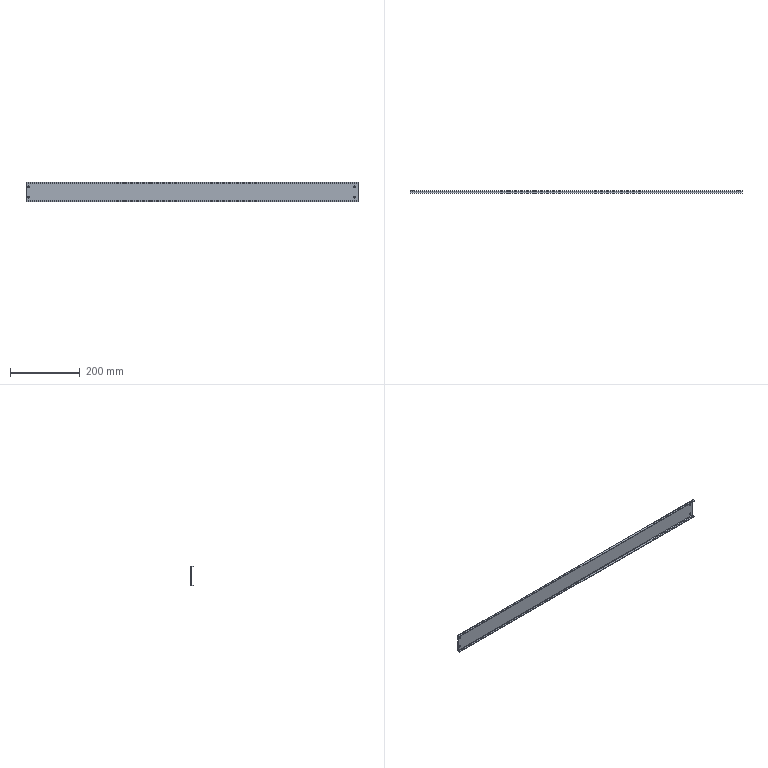Part | STEP file | 866-BDO024-95-03A | 1 solid | 22 faces | box 954 x 8 x 56 mm | volume 95867 mm3 | cylinder 12 | plane 10 | commonest cylinder face diameters 4.8 x8 3 x2 6 x2
STEP:
#1=CARTESIAN_POINT('',(944.,-1.5,12.6));
#2=VERTEX_POINT('',#1);
#3=CARTESIAN_POINT('',(944.,-1.5,17.4));
#4=VERTEX_POINT('',#3);
#5=CARTESIAN_POINT('',(944.,-1.5,15.));
#6=DIRECTION('',(0.,1.,0.));
#7=DIRECTION('',(0.,0.,1.));
#8=AXIS2_PLACEMENT_3D('',#5,#6,#7);
#9=CIRCLE('',#8,2.4);
#10=EDGE_CURVE('',#2,#4,#9,.T.);
#11=ORIENTED_EDGE('',*,*,#10,.F.);
#12=CARTESIAN_POINT('',(944.,0.,12.6));
#13=VERTEX_POINT('',#12);
#14=CARTESIAN_POINT('',(944.,0.,12.6));
#15=DIRECTION('',(0.,1.,0.));
#16=VECTOR('',#15,1000.);
#17=LINE('',#14,#16);
#18=EDGE_CURVE('',#2,#13,#17,.T.);
#19=ORIENTED_EDGE('',*,*,#18,.T.);
#20=CARTESIAN_POINT('',(944.,0.,17.4));
#21=VERTEX_POINT('',#20);
#22=CARTESIAN_POINT('',(944.,0.,15.));
#23=DIRECTION('',(0.,-1.,0.));
#24=DIRECTION('',(0.,0.,1.));
#25=AXIS2_PLACEMENT_3D('',#22,#23,#24);
#26=CIRCLE('',#25,2.4);
#27=EDGE_CURVE('',#21,#13,#26,.T.);
#28=ORIENTED_EDGE('',*,*,#27,.F.);
#29=CARTESIAN_POINT('',(944.,0.,17.4));
#30=DIRECTION('',(0.,1.,0.));
#31=VECTOR('',#30,1000.);
#32=LINE('',#29,#31);
#33=EDGE_CURVE('',#4,#21,#32,.T.);
#34=ORIENTED_EDGE('',*,*,#33,.F.);
#35=EDGE_LOOP('',(#11,#19,#28,#34));
#36=FACE_OUTER_BOUND('',#35,.T.);
#37=CARTESIAN_POINT('',(944.,0.,15.));
#38=DIRECTION('',(0.,1.,0.));
#39=DIRECTION('',(0.,0.,1.));
#40=AXIS2_PLACEMENT_3D('',#37,#38,#39);
#41=CYLINDRICAL_SURFACE('',#40,2.4);
#42=ADVANCED_FACE('',(#36),#41,.F.);
#43=CARTESIAN_POINT('',(944.,-1.5,-17.4));
#44=VERTEX_POINT('',#43);
#45=CARTESIAN_POINT('',(944.,-1.5,-12.6));
#46=VERTEX_POINT('',#45);
#47=CARTESIAN_POINT('',(944.,-1.5,-15.));
#48=DIRECTION('',(0.,1.,0.));
#49=DIRECTION('',(0.,0.,1.));
#50=AXIS2_PLACEMENT_3D('',#47,#48,#49);
#51=CIRCLE('',#50,2.4);
#52=EDGE_CURVE('',#44,#46,#51,.T.);
#53=ORIENTED_EDGE('',*,*,#52,.F.);
#54=CARTESIAN_POINT('',(944.,0.,-17.4));
#55=VERTEX_POINT('',#54);
#56=CARTESIAN_POINT('',(944.,0.,-17.4));
#57=DIRECTION('',(0.,1.,0.));
#58=VECTOR('',#57,1000.);
#59=LINE('',#56,#58);
#60=EDGE_CURVE('',#44,#55,#59,.T.);
#61=ORIENTED_EDGE('',*,*,#60,.T.);
#62=CARTESIAN_POINT('',(944.,0.,-12.6));
#63=VERTEX_POINT('',#62);
#64=CARTESIAN_POINT('',(944.,0.,-15.));
#65=DIRECTION('',(0.,-1.,0.));
#66=DIRECTION('',(0.,0.,1.));
#67=AXIS2_PLACEMENT_3D('',#64,#65,#66);
#68=CIRCLE('',#67,2.4);
#69=EDGE_CURVE('',#63,#55,#68,.T.);
#70=ORIENTED_EDGE('',*,*,#69,.F.);
#71=CARTESIAN_POINT('',(944.,0.,-12.6));
#72=DIRECTION('',(0.,1.,0.));
#73=VECTOR('',#72,1000.);
#74=LINE('',#71,#73);
#75=EDGE_CURVE('',#46,#63,#74,.T.);
#76=ORIENTED_EDGE('',*,*,#75,.F.);
#77=EDGE_LOOP('',(#53,#61,#70,#76));
#78=FACE_OUTER_BOUND('',#77,.T.);
#79=CARTESIAN_POINT('',(944.,0.,-15.));
#80=DIRECTION('',(0.,1.,0.));
#81=DIRECTION('',(0.,0.,1.));
#82=AXIS2_PLACEMENT_3D('',#79,#80,#81);
#83=CYLINDRICAL_SURFACE('',#82,2.4);
#84=ADVANCED_FACE('',(#78),#83,.F.);
#85=CARTESIAN_POINT('',(7.,-1.5,-17.4));
#86=VERTEX_POINT('',#85);
#87=CARTESIAN_POINT('',(7.,-1.5,-12.6));
#88=VERTEX_POINT('',#87);
#89=CARTESIAN_POINT('',(7.,-1.5,-15.));
#90=DIRECTION('',(0.,1.,0.));
#91=DIRECTION('',(0.,0.,1.));
#92=AXIS2_PLACEMENT_3D('',#89,#90,#91);
#93=CIRCLE('',#92,2.4);
#94=EDGE_CURVE('',#86,#88,#93,.T.);
#95=ORIENTED_EDGE('',*,*,#94,.F.);
#96=CARTESIAN_POINT('',(7.,0.,-17.4));
#97=VERTEX_POINT('',#96);
#98=CARTESIAN_POINT('',(7.,0.,-17.4));
#99=DIRECTION('',(0.,1.,0.));
#100=VECTOR('',#99,1000.);
#101=LINE('',#98,#100);
#102=EDGE_CURVE('',#86,#97,#101,.T.);
#103=ORIENTED_EDGE('',*,*,#102,.T.);
#104=CARTESIAN_POINT('',(7.,0.,-12.6));
#105=VERTEX_POINT('',#104);
#106=CARTESIAN_POINT('',(7.,0.,-15.));
#107=DIRECTION('',(0.,-1.,0.));
#108=DIRECTION('',(0.,0.,1.));
#109=AXIS2_PLACEMENT_3D('',#106,#107,#108);
#110=CIRCLE('',#109,2.4);
#111=EDGE_CURVE('',#105,#97,#110,.T.);
#112=ORIENTED_EDGE('',*,*,#111,.F.);
#113=CARTESIAN_POINT('',(7.,0.,-12.6));
#114=DIRECTION('',(0.,1.,0.));
#115=VECTOR('',#114,1000.);
#116=LINE('',#113,#115);
#117=EDGE_CURVE('',#88,#105,#116,.T.);
#118=ORIENTED_EDGE('',*,*,#117,.F.);
#119=EDGE_LOOP('',(#95,#103,#112,#118));
#120=FACE_OUTER_BOUND('',#119,.T.);
#121=CARTESIAN_POINT('',(7.,0.,-15.));
#122=DIRECTION('',(0.,1.,0.));
#123=DIRECTION('',(0.,0.,1.));
#124=AXIS2_PLACEMENT_3D('',#121,#122,#123);
#125=CYLINDRICAL_SURFACE('',#124,2.4);
#126=ADVANCED_FACE('',(#120),#125,.F.);
#127=CARTESIAN_POINT('',(7.,-1.5,12.6));
#128=VERTEX_POINT('',#127);
#129=CARTESIAN_POINT('',(7.,-1.5,17.4));
#130=VERTEX_POINT('',#129);
#131=CARTESIAN_POINT('',(7.,-1.5,15.));
#132=DIRECTION('',(0.,1.,0.));
#133=DIRECTION('',(0.,0.,1.));
#134=AXIS2_PLACEMENT_3D('',#131,#132,#133);
#135=CIRCLE('',#134,2.4);
#136=EDGE_CURVE('',#128,#130,#135,.T.);
#137=ORIENTED_EDGE('',*,*,#136,.F.);
#138=CARTESIAN_POINT('',(7.,0.,12.6));
#139=VERTEX_POINT('',#138);
#140=CARTESIAN_POINT('',(7.,0.,12.6));
#141=DIRECTION('',(0.,1.,0.));
#142=VECTOR('',#141,1000.);
#143=LINE('',#140,#142);
#144=EDGE_CURVE('',#128,#139,#143,.T.);
#145=ORIENTED_EDGE('',*,*,#144,.T.);
#146=CARTESIAN_POINT('',(7.,0.,17.4));
#147=VERTEX_POINT('',#146);
#148=CARTESIAN_POINT('',(7.,0.,15.));
#149=DIRECTION('',(0.,-1.,0.));
#150=DIRECTION('',(0.,0.,1.));
#151=AXIS2_PLACEMENT_3D('',#148,#149,#150);
#152=CIRCLE('',#151,2.4);
#153=EDGE_CURVE('',#147,#139,#152,.T.);
#154=ORIENTED_EDGE('',*,*,#153,.F.);
#155=CARTESIAN_POINT('',(7.,0.,17.4));
#156=DIRECTION('',(0.,1.,0.));
#157=VECTOR('',#156,1000.);
#158=LINE('',#155,#157);
#159=EDGE_CURVE('',#130,#147,#158,.T.);
#160=ORIENTED_EDGE('',*,*,#159,.F.);
#161=EDGE_LOOP('',(#137,#145,#154,#160));
#162=FACE_OUTER_BOUND('',#161,.T.);
#163=CARTESIAN_POINT('',(7.,0.,15.));
#164=DIRECTION('',(0.,1.,0.));
#165=DIRECTION('',(0.,0.,1.));
#166=AXIS2_PLACEMENT_3D('',#163,#164,#165);
#167=CYLINDRICAL_SURFACE('',#166,2.4);
#168=ADVANCED_FACE('',(#162),#167,.F.);
#169=CARTESIAN_POINT('',(954.,0.,25.));
#170=VERTEX_POINT('',#169);
#171=CARTESIAN_POINT('',(954.,0.,-25.));
#172=VERTEX_POINT('',#171);
#173=CARTESIAN_POINT('',(954.,0.,28.));
#174=DIRECTION('',(0.,0.,-1.));
#175=VECTOR('',#174,1000.);
#176=LINE('',#173,#175);
#177=EDGE_CURVE('',#170,#172,#176,.T.);
#178=ORIENTED_EDGE('',*,*,#177,.T.);
#179=CARTESIAN_POINT('',(0.,0.,-25.));
#180=VERTEX_POINT('',#179);
#181=CARTESIAN_POINT('',(954.,0.,-25.));
#182=DIRECTION('',(-1.,0.,0.));
#183=VECTOR('',#182,1000.);
#184=LINE('',#181,#183);
#185=EDGE_CURVE('',#172,#180,#184,.T.);
#186=ORIENTED_EDGE('',*,*,#185,.T.);
#187=CARTESIAN_POINT('',(0.,0.,25.));
#188=VERTEX_POINT('',#187);
#189=CARTESIAN_POINT('',(0.,0.,28.));
#190=DIRECTION('',(0.,0.,1.));
#191=VECTOR('',#190,1000.);
#192=LINE('',#189,#191);
#193=EDGE_CURVE('',#180,#188,#192,.T.);
#194=ORIENTED_EDGE('',*,*,#193,.T.);
#195=CARTESIAN_POINT('',(954.,0.,25.));
#196=DIRECTION('',(1.,0.,0.));
#197=VECTOR('',#196,1000.);
#198=LINE('',#195,#197);
#199=EDGE_CURVE('',#188,#170,#198,.T.);
#200=ORIENTED_EDGE('',*,*,#199,.T.);
#201=EDGE_LOOP('',(#178,#186,#194,#200));
#202=FACE_OUTER_BOUND('',#201,.T.);
#203=ORIENTED_EDGE('',*,*,#27,.T.);
#204=CARTESIAN_POINT('',(944.,0.,15.));
#205=DIRECTION('',(0.,-1.,0.));
#206=DIRECTION('',(0.,0.,1.));
#207=AXIS2_PLACEMENT_3D('',#204,#205,#206);
#208=CIRCLE('',#207,2.4);
#209=EDGE_CURVE('',#13,#21,#208,.T.);
#210=ORIENTED_EDGE('',*,*,#209,.T.);
#211=EDGE_LOOP('',(#203,#210));
#212=FACE_BOUND('',#211,.T.);
#213=ORIENTED_EDGE('',*,*,#69,.T.);
#214=CARTESIAN_POINT('',(944.,0.,-15.));
#215=DIRECTION('',(0.,-1.,0.));
#216=DIRECTION('',(0.,0.,1.));
#217=AXIS2_PLACEMENT_3D('',#214,#215,#216);
#218=CIRCLE('',#217,2.4);
#219=EDGE_CURVE('',#55,#63,#218,.T.);
#220=ORIENTED_EDGE('',*,*,#219,.T.);
#221=EDGE_LOOP('',(#213,#220));
#222=FACE_BOUND('',#221,.T.);
#223=ORIENTED_EDGE('',*,*,#111,.T.);
#224=CARTESIAN_POINT('',(7.,0.,-15.));
#225=DIRECTION('',(0.,-1.,0.));
#226=DIRECTION('',(0.,0.,1.));
#227=AXIS2_PLACEMENT_3D('',#224,#225,#226);
#228=CIRCLE('',#227,2.4);
#229=EDGE_CURVE('',#97,#105,#228,.T.);
#230=ORIENTED_EDGE('',*,*,#229,.T.);
#231=EDGE_LOOP('',(#223,#230));
#232=FACE_BOUND('',#231,.T.);
#233=ORIENTED_EDGE('',*,*,#153,.T.);
#234=CARTESIAN_POINT('',(7.,0.,15.));
#235=DIRECTION('',(0.,-1.,0.));
#236=DIRECTION('',(0.,0.,1.));
#237=AXIS2_PLACEMENT_3D('',#234,#235,#236);
#238=CIRCLE('',#237,2.4);
#239=EDGE_CURVE('',#139,#147,#238,.T.);
#240=ORIENTED_EDGE('',*,*,#239,.T.);
#241=EDGE_LOOP('',(#233,#240));
#242=FACE_BOUND('',#241,.T.);
#243=CARTESIAN_POINT('',(954.,0.,28.));
#244=DIRECTION('',(0.,1.,0.));
#245=DIRECTION('',(0.,0.,1.));
#246=AXIS2_PLACEMENT_3D('',#243,#244,#245);
#247=PLANE('',#246);
#248=ADVANCED_FACE('',(#202,#212,#222,#232,#242),#247,.T.);
#249=CARTESIAN_POINT('',(954.,-3.,-28.));
#250=VERTEX_POINT('',#249);
#251=CARTESIAN_POINT('',(954.,-3.,-25.));
#252=DIRECTION('',(-1.,0.,0.));
#253=DIRECTION('',(0.,0.,1.));
#254=AXIS2_PLACEMENT_3D('',#251,#252,#253);
#255=CIRCLE('',#254,3.);
#256=EDGE_CURVE('',#172,#250,#255,.T.);
#257=ORIENTED_EDGE('',*,*,#256,.T.);
#258=CARTESIAN_POINT('',(0.,-3.,-28.));
#259=VERTEX_POINT('',#258);
#260=CARTESIAN_POINT('',(954.,-3.,-28.));
#261=DIRECTION('',(-1.,0.,0.));
#262=VECTOR('',#261,1000.);
#263=LINE('',#260,#262);
#264=EDGE_CURVE('',#250,#259,#263,.T.);
#265=ORIENTED_EDGE('',*,*,#264,.T.);
#266=CARTESIAN_POINT('',(0.,-3.,-25.));
#267=DIRECTION('',(1.,0.,0.));
#268=DIRECTION('',(0.,0.,1.));
#269=AXIS2_PLACEMENT_3D('',#266,#267,#268);
#270=CIRCLE('',#269,3.);
#271=EDGE_CURVE('',#259,#180,#270,.T.);
#272=ORIENTED_EDGE('',*,*,#271,.T.);
#273=ORIENTED_EDGE('',*,*,#185,.F.);
#274=EDGE_LOOP('',(#257,#265,#272,#273));
#275=FACE_OUTER_BOUND('',#274,.T.);
#276=CARTESIAN_POINT('',(954.,-3.,-25.));
#277=DIRECTION('',(-1.,0.,0.));
#278=DIRECTION('',(0.,0.,1.));
#279=AXIS2_PLACEMENT_3D('',#276,#277,#278);
#280=CYLINDRICAL_SURFACE('',#279,3.);
#281=ADVANCED_FACE('',(#275),#280,.T.);
#282=CARTESIAN_POINT('',(954.,-1.5,25.));
#283=VERTEX_POINT('',#282);
#284=CARTESIAN_POINT('',(954.,-1.5,-25.));
#285=VERTEX_POINT('',#284);
#286=CARTESIAN_POINT('',(954.,-1.5,26.5));
#287=DIRECTION('',(0.,0.,-1.));
#288=VECTOR('',#287,1000.);
#289=LINE('',#286,#288);
#290=EDGE_CURVE('',#283,#285,#289,.T.);
#291=ORIENTED_EDGE('',*,*,#290,.T.);
#292=CARTESIAN_POINT('',(954.,-3.,-26.5));
#293=VERTEX_POINT('',#292);
#294=CARTESIAN_POINT('',(954.,-3.,-25.));
#295=DIRECTION('',(-1.,0.,0.));
#296=DIRECTION('',(0.,0.,1.));
#297=AXIS2_PLACEMENT_3D('',#294,#295,#296);
#298=CIRCLE('',#297,1.5);
#299=EDGE_CURVE('',#285,#293,#298,.T.);
#300=ORIENTED_EDGE('',*,*,#299,.T.);
#301=CARTESIAN_POINT('',(954.,-8.,-26.5));
#302=VERTEX_POINT('',#301);
#303=CARTESIAN_POINT('',(954.,-1.5,-26.5));
#304=DIRECTION('',(0.,-1.,0.));
#305=VECTOR('',#304,1000.);
#306=LINE('',#303,#305);
#307=EDGE_CURVE('',#293,#302,#306,.T.);
#308=ORIENTED_EDGE('',*,*,#307,.T.);
#309=CARTESIAN_POINT('',(954.,-8.,-28.));
#310=VERTEX_POINT('',#309);
#311=CARTESIAN_POINT('',(954.,-8.,-28.));
#312=DIRECTION('',(0.,0.,1.));
#313=VECTOR('',#312,1000.);
#314=LINE('',#311,#313);
#315=EDGE_CURVE('',#310,#302,#314,.T.);
#316=ORIENTED_EDGE('',*,*,#315,.F.);
#317=CARTESIAN_POINT('',(954.,0.,-28.));
#318=DIRECTION('',(0.,-1.,0.));
#319=VECTOR('',#318,1000.);
#320=LINE('',#317,#319);
#321=EDGE_CURVE('',#250,#310,#320,.T.);
#322=ORIENTED_EDGE('',*,*,#321,.F.);
#323=ORIENTED_EDGE('',*,*,#256,.F.);
#324=ORIENTED_EDGE('',*,*,#177,.F.);
#325=CARTESIAN_POINT('',(954.,-3.,28.));
#326=VERTEX_POINT('',#325);
#327=CARTESIAN_POINT('',(954.,-3.,25.));
#328=DIRECTION('',(-1.,0.,0.));
#329=DIRECTION('',(0.,0.,1.));
#330=AXIS2_PLACEMENT_3D('',#327,#328,#329);
#331=CIRCLE('',#330,3.);
#332=EDGE_CURVE('',#326,#170,#331,.T.);
#333=ORIENTED_EDGE('',*,*,#332,.F.);
#334=CARTESIAN_POINT('',(954.,-8.,28.));
#335=VERTEX_POINT('',#334);
#336=CARTESIAN_POINT('',(954.,-8.,28.));
#337=DIRECTION('',(0.,1.,0.));
#338=VECTOR('',#337,1000.);
#339=LINE('',#336,#338);
#340=EDGE_CURVE('',#335,#326,#339,.T.);
#341=ORIENTED_EDGE('',*,*,#340,.F.);
#342=CARTESIAN_POINT('',(954.,-8.,26.5));
#343=VERTEX_POINT('',#342);
#344=CARTESIAN_POINT('',(954.,-8.,-25.));
#345=DIRECTION('',(0.,0.,-1.));
#346=VECTOR('',#345,1000.);
#347=LINE('',#344,#346);
#348=EDGE_CURVE('',#335,#343,#347,.T.);
#349=ORIENTED_EDGE('',*,*,#348,.T.);
#350=CARTESIAN_POINT('',(954.,-3.,26.5));
#351=VERTEX_POINT('',#350);
#352=CARTESIAN_POINT('',(954.,-3.,26.5));
#353=DIRECTION('',(0.,1.,0.));
#354=VECTOR('',#353,1000.);
#355=LINE('',#352,#354);
#356=EDGE_CURVE('',#343,#351,#355,.T.);
#357=ORIENTED_EDGE('',*,*,#356,.T.);
#358=CARTESIAN_POINT('',(954.,-3.,25.));
#359=DIRECTION('',(-1.,0.,0.));
#360=DIRECTION('',(0.,0.,1.));
#361=AXIS2_PLACEMENT_3D('',#358,#359,#360);
#362=CIRCLE('',#361,1.5);
#363=EDGE_CURVE('',#351,#283,#362,.T.);
#364=ORIENTED_EDGE('',*,*,#363,.T.);
#365=EDGE_LOOP('',(#291,#300,#308,#316,#322,#323,#324,#333,#341,#349,#357,#364));
#366=FACE_OUTER_BOUND('',#365,.T.);
#367=CARTESIAN_POINT('',(954.,-3.,26.5));
#368=DIRECTION('',(1.,0.,0.));
#369=DIRECTION('',(0.,0.,-1.));
#370=AXIS2_PLACEMENT_3D('',#367,#368,#369);
#371=PLANE('',#370);
#372=ADVANCED_FACE('',(#366),#371,.T.);
#373=ORIENTED_EDGE('',*,*,#332,.T.);
#374=ORIENTED_EDGE('',*,*,#199,.F.);
#375=CARTESIAN_POINT('',(0.,-3.,28.));
#376=VERTEX_POINT('',#375);
#377=CARTESIAN_POINT('',(0.,-3.,25.));
#378=DIRECTION('',(1.,0.,0.));
#379=DIRECTION('',(0.,0.,1.));
#380=AXIS2_PLACEMENT_3D('',#377,#378,#379);
#381=CIRCLE('',#380,3.);
#382=EDGE_CURVE('',#188,#376,#381,.T.);
#383=ORIENTED_EDGE('',*,*,#382,.T.);
#384=CARTESIAN_POINT('',(954.,-3.,28.));
#385=DIRECTION('',(1.,0.,0.));
#386=VECTOR('',#385,1000.);
#387=LINE('',#384,#386);
#388=EDGE_CURVE('',#376,#326,#387,.T.);
#389=ORIENTED_EDGE('',*,*,#388,.T.);
#390=EDGE_LOOP('',(#373,#374,#383,#389));
#391=FACE_OUTER_BOUND('',#390,.T.);
#392=CARTESIAN_POINT('',(954.,-3.,25.));
#393=DIRECTION('',(-1.,0.,0.));
#394=DIRECTION('',(0.,0.,1.));
#395=AXIS2_PLACEMENT_3D('',#392,#393,#394);
#396=CYLINDRICAL_SURFACE('',#395,3.);
#397=ADVANCED_FACE('',(#391),#396,.T.);
#398=CARTESIAN_POINT('',(0.,-1.5,-25.));
#399=VERTEX_POINT('',#398);
#400=CARTESIAN_POINT('',(0.,-1.5,25.));
#401=VERTEX_POINT('',#400);
#402=CARTESIAN_POINT('',(0.,-1.5,-26.5));
#403=DIRECTION('',(0.,0.,1.));
#404=VECTOR('',#403,1000.);
#405=LINE('',#402,#404);
#406=EDGE_CURVE('',#399,#401,#405,.T.);
#407=ORIENTED_EDGE('',*,*,#406,.T.);
#408=CARTESIAN_POINT('',(0.,-3.,26.5));
#409=VERTEX_POINT('',#408);
#410=CARTESIAN_POINT('',(0.,-3.,25.));
#411=DIRECTION('',(1.,0.,0.));
#412=DIRECTION('',(0.,0.,1.));
#413=AXIS2_PLACEMENT_3D('',#410,#411,#412);
#414=CIRCLE('',#413,1.5);
#415=EDGE_CURVE('',#401,#409,#414,.T.);
#416=ORIENTED_EDGE('',*,*,#415,.T.);
#417=CARTESIAN_POINT('',(0.,-8.,26.5));
#418=VERTEX_POINT('',#417);
#419=CARTESIAN_POINT('',(0.,-1.5,26.5));
#420=DIRECTION('',(0.,-1.,0.));
#421=VECTOR('',#420,1000.);
#422=LINE('',#419,#421);
#423=EDGE_CURVE('',#409,#418,#422,.T.);
#424=ORIENTED_EDGE('',*,*,#423,.T.);
#425=CARTESIAN_POINT('',(0.,-8.,28.));
#426=VERTEX_POINT('',#425);
#427=CARTESIAN_POINT('',(0.,-8.,26.5));
#428=DIRECTION('',(0.,0.,-1.));
#429=VECTOR('',#428,1000.);
#430=LINE('',#427,#429);
#431=EDGE_CURVE('',#426,#418,#430,.T.);
#432=ORIENTED_EDGE('',*,*,#431,.F.);
#433=CARTESIAN_POINT('',(0.,-8.,28.));
#434=DIRECTION('',(0.,-1.,0.));
#435=VECTOR('',#434,1000.);
#436=LINE('',#433,#435);
#437=EDGE_CURVE('',#376,#426,#436,.T.);
#438=ORIENTED_EDGE('',*,*,#437,.F.);
#439=ORIENTED_EDGE('',*,*,#382,.F.);
#440=ORIENTED_EDGE('',*,*,#193,.F.);
#441=ORIENTED_EDGE('',*,*,#271,.F.);
#442=CARTESIAN_POINT('',(0.,-8.,-28.));
#443=VERTEX_POINT('',#442);
#444=CARTESIAN_POINT('',(0.,0.,-28.));
#445=DIRECTION('',(0.,1.,0.));
#446=VECTOR('',#445,1000.);
#447=LINE('',#444,#446);
#448=EDGE_CURVE('',#443,#259,#447,.T.);
#449=ORIENTED_EDGE('',*,*,#448,.F.);
#450=CARTESIAN_POINT('',(0.,-8.,-26.5));
#451=VERTEX_POINT('',#450);
#452=CARTESIAN_POINT('',(0.,-8.,-28.));
#453=DIRECTION('',(0.,0.,-1.));
#454=VECTOR('',#453,1000.);
#455=LINE('',#452,#454);
#456=EDGE_CURVE('',#451,#443,#455,.T.);
#457=ORIENTED_EDGE('',*,*,#456,.F.);
#458=CARTESIAN_POINT('',(0.,-3.,-26.5));
#459=VERTEX_POINT('',#458);
#460=CARTESIAN_POINT('',(0.,-3.,-26.5));
#461=DIRECTION('',(0.,-1.,0.));
#462=VECTOR('',#461,1000.);
#463=LINE('',#460,#462);
#464=EDGE_CURVE('',#459,#451,#463,.T.);
#465=ORIENTED_EDGE('',*,*,#464,.F.);
#466=CARTESIAN_POINT('',(0.,-3.,-25.));
#467=DIRECTION('',(1.,0.,0.));
#468=DIRECTION('',(0.,0.,1.));
#469=AXIS2_PLACEMENT_3D('',#466,#467,#468);
#470=CIRCLE('',#469,1.5);
#471=EDGE_CURVE('',#459,#399,#470,.T.);
#472=ORIENTED_EDGE('',*,*,#471,.T.);
#473=EDGE_LOOP('',(#407,#416,#424,#432,#438,#439,#440,#441,#449,#457,#465,#472));
#474=FACE_OUTER_BOUND('',#473,.T.);
#475=CARTESIAN_POINT('',(0.,-3.,-26.5));
#476=DIRECTION('',(-1.,0.,0.));
#477=DIRECTION('',(0.,0.,1.));
#478=AXIS2_PLACEMENT_3D('',#475,#476,#477);
#479=PLANE('',#478);
#480=ADVANCED_FACE('',(#474),#479,.T.);
#481=ORIENTED_EDGE('',*,*,#18,.F.);
#482=CARTESIAN_POINT('',(944.,-1.5,15.));
#483=DIRECTION('',(0.,1.,0.));
#484=DIRECTION('',(0.,0.,1.));
#485=AXIS2_PLACEMENT_3D('',#482,#483,#484);
#486=CIRCLE('',#485,2.4);
#487=EDGE_CURVE('',#4,#2,#486,.T.);
#488=ORIENTED_EDGE('',*,*,#487,.F.);
#489=ORIENTED_EDGE('',*,*,#33,.T.);
#490=ORIENTED_EDGE('',*,*,#209,.F.);
#491=EDGE_LOOP('',(#481,#488,#489,#490));
#492=FACE_OUTER_BOUND('',#491,.T.);
#493=CARTESIAN_POINT('',(944.,0.,15.));
#494=DIRECTION('',(0.,1.,0.));
#495=DIRECTION('',(0.,0.,1.));
#496=AXIS2_PLACEMENT_3D('',#493,#494,#495);
#497=CYLINDRICAL_SURFACE('',#496,2.4);
#498=ADVANCED_FACE('',(#492),#497,.F.);
#499=ORIENTED_EDGE('',*,*,#60,.F.);
#500=CARTESIAN_POINT('',(944.,-1.5,-15.));
#501=DIRECTION('',(0.,1.,0.));
#502=DIRECTION('',(0.,0.,1.));
#503=AXIS2_PLACEMENT_3D('',#500,#501,#502);
#504=CIRCLE('',#503,2.4);
#505=EDGE_CURVE('',#46,#44,#504,.T.);
#506=ORIENTED_EDGE('',*,*,#505,.F.);
#507=ORIENTED_EDGE('',*,*,#75,.T.);
#508=ORIENTED_EDGE('',*,*,#219,.F.);
#509=EDGE_LOOP('',(#499,#506,#507,#508));
#510=FACE_OUTER_BOUND('',#509,.T.);
#511=CARTESIAN_POINT('',(944.,0.,-15.));
#512=DIRECTION('',(0.,1.,0.));
#513=DIRECTION('',(0.,0.,1.));
#514=AXIS2_PLACEMENT_3D('',#511,#512,#513);
#515=CYLINDRICAL_SURFACE('',#514,2.4);
#516=ADVANCED_FACE('',(#510),#515,.F.);
#517=ORIENTED_EDGE('',*,*,#102,.F.);
#518=CARTESIAN_POINT('',(7.,-1.5,-15.));
#519=DIRECTION('',(0.,1.,0.));
#520=DIRECTION('',(0.,0.,1.));
#521=AXIS2_PLACEMENT_3D('',#518,#519,#520);
#522=CIRCLE('',#521,2.4);
#523=EDGE_CURVE('',#88,#86,#522,.T.);
#524=ORIENTED_EDGE('',*,*,#523,.F.);
#525=ORIENTED_EDGE('',*,*,#117,.T.);
#526=ORIENTED_EDGE('',*,*,#229,.F.);
#527=EDGE_LOOP('',(#517,#524,#525,#526));
#528=FACE_OUTER_BOUND('',#527,.T.);
#529=CARTESIAN_POINT('',(7.,0.,-15.));
#530=DIRECTION('',(0.,1.,0.));
#531=DIRECTION('',(0.,0.,1.));
#532=AXIS2_PLACEMENT_3D('',#529,#530,#531);
#533=CYLINDRICAL_SURFACE('',#532,2.4);
#534=ADVANCED_FACE('',(#528),#533,.F.);
#535=ORIENTED_EDGE('',*,*,#144,.F.);
#536=CARTESIAN_POINT('',(7.,-1.5,15.));
#537=DIRECTION('',(0.,1.,0.));
#538=DIRECTION('',(0.,0.,1.));
#539=AXIS2_PLACEMENT_3D('',#536,#537,#538);
#540=CIRCLE('',#539,2.4);
#541=EDGE_CURVE('',#130,#128,#540,.T.);
#542=ORIENTED_EDGE('',*,*,#541,.F.);
#543=ORIENTED_EDGE('',*,*,#159,.T.);
#544=ORIENTED_EDGE('',*,*,#239,.F.);
#545=EDGE_LOOP('',(#535,#542,#543,#544));
#546=FACE_OUTER_BOUND('',#545,.T.);
#547=CARTESIAN_POINT('',(7.,0.,15.));
#548=DIRECTION('',(0.,1.,0.));
#549=DIRECTION('',(0.,0.,1.));
#550=AXIS2_PLACEMENT_3D('',#547,#548,#549);
#551=CYLINDRICAL_SURFACE('',#550,2.4);
#552=ADVANCED_FACE('',(#546),#551,.F.);
#553=ORIENTED_EDGE('',*,*,#321,.T.);
#554=CARTESIAN_POINT('',(954.,-8.,-28.));
#555=DIRECTION('',(-1.,0.,0.));
#556=VECTOR('',#555,1000.);
#557=LINE('',#554,#556);
#558=EDGE_CURVE('',#310,#443,#557,.T.);
#559=ORIENTED_EDGE('',*,*,#558,.T.);
#560=ORIENTED_EDGE('',*,*,#448,.T.);
#561=ORIENTED_EDGE('',*,*,#264,.F.);
#562=EDGE_LOOP('',(#553,#559,#560,#561));
#563=FACE_OUTER_BOUND('',#562,.T.);
#564=CARTESIAN_POINT('',(954.,0.,-28.));
#565=DIRECTION('',(0.,0.,-1.));
#566=DIRECTION('',(-1.,0.,0.));
#567=AXIS2_PLACEMENT_3D('',#564,#565,#566);
#568=PLANE('',#567);
#569=ADVANCED_FACE('',(#563),#568,.T.);
#570=CARTESIAN_POINT('',(954.,-1.5,-25.));
#571=DIRECTION('',(-1.,0.,0.));
#572=VECTOR('',#571,1000.);
#573=LINE('',#570,#572);
#574=EDGE_CURVE('',#285,#399,#573,.T.);
#575=ORIENTED_EDGE('',*,*,#574,.F.);
#576=ORIENTED_EDGE('',*,*,#290,.F.);
#577=CARTESIAN_POINT('',(954.,-1.5,25.));
#578=DIRECTION('',(1.,0.,0.));
#579=VECTOR('',#578,1000.);
#580=LINE('',#577,#579);
#581=EDGE_CURVE('',#401,#283,#580,.T.);
#582=ORIENTED_EDGE('',*,*,#581,.F.);
#583=ORIENTED_EDGE('',*,*,#406,.F.);
#584=EDGE_LOOP('',(#575,#576,#582,#583));
#585=FACE_OUTER_BOUND('',#584,.T.);
#586=ORIENTED_EDGE('',*,*,#487,.T.);
#587=ORIENTED_EDGE('',*,*,#10,.T.);
#588=EDGE_LOOP('',(#586,#587));
#589=FACE_BOUND('',#588,.T.);
#590=ORIENTED_EDGE('',*,*,#505,.T.);
#591=ORIENTED_EDGE('',*,*,#52,.T.);
#592=EDGE_LOOP('',(#590,#591));
#593=FACE_BOUND('',#592,.T.);
#594=ORIENTED_EDGE('',*,*,#523,.T.);
#595=ORIENTED_EDGE('',*,*,#94,.T.);
#596=EDGE_LOOP('',(#594,#595));
#597=FACE_BOUND('',#596,.T.);
#598=ORIENTED_EDGE('',*,*,#541,.T.);
#599=ORIENTED_EDGE('',*,*,#136,.T.);
#600=EDGE_LOOP('',(#598,#599));
#601=FACE_BOUND('',#600,.T.);
#602=CARTESIAN_POINT('',(954.,-1.5,28.));
#603=DIRECTION('',(0.,1.,0.));
#604=DIRECTION('',(0.,0.,1.));
#605=AXIS2_PLACEMENT_3D('',#602,#603,#604);
#606=PLANE('',#605);
#607=ADVANCED_FACE('',(#585,#589,#593,#597,#601),#606,.F.);
#608=ORIENTED_EDGE('',*,*,#340,.T.);
#609=ORIENTED_EDGE('',*,*,#388,.F.);
#610=ORIENTED_EDGE('',*,*,#437,.T.);
#611=CARTESIAN_POINT('',(954.,-8.,28.));
#612=DIRECTION('',(1.,0.,0.));
#613=VECTOR('',#612,1000.);
#614=LINE('',#611,#613);
#615=EDGE_CURVE('',#426,#335,#614,.T.);
#616=ORIENTED_EDGE('',*,*,#615,.T.);
#617=EDGE_LOOP('',(#608,#609,#610,#616));
#618=FACE_OUTER_BOUND('',#617,.T.);
#619=CARTESIAN_POINT('',(954.,-8.,28.));
#620=DIRECTION('',(0.,0.,1.));
#621=DIRECTION('',(1.,0.,0.));
#622=AXIS2_PLACEMENT_3D('',#619,#620,#621);
#623=PLANE('',#622);
#624=ADVANCED_FACE('',(#618),#623,.T.);
#625=ORIENTED_EDGE('',*,*,#315,.T.);
#626=CARTESIAN_POINT('',(954.,-8.,-26.5));
#627=DIRECTION('',(-1.,0.,0.));
#628=VECTOR('',#627,1000.);
#629=LINE('',#626,#628);
#630=EDGE_CURVE('',#302,#451,#629,.T.);
#631=ORIENTED_EDGE('',*,*,#630,.T.);
#632=ORIENTED_EDGE('',*,*,#456,.T.);
#633=ORIENTED_EDGE('',*,*,#558,.F.);
#634=EDGE_LOOP('',(#625,#631,#632,#633));
#635=FACE_OUTER_BOUND('',#634,.T.);
#636=CARTESIAN_POINT('',(954.,-8.,-28.));
#637=DIRECTION('',(0.,-1.,0.));
#638=DIRECTION('',(0.,0.,-1.));
#639=AXIS2_PLACEMENT_3D('',#636,#637,#638);
#640=PLANE('',#639);
#641=ADVANCED_FACE('',(#635),#640,.T.);
#642=CARTESIAN_POINT('',(954.,-3.,-26.5));
#643=DIRECTION('',(-1.,0.,0.));
#644=VECTOR('',#643,1000.);
#645=LINE('',#642,#644);
#646=EDGE_CURVE('',#293,#459,#645,.T.);
#647=ORIENTED_EDGE('',*,*,#646,.F.);
#648=ORIENTED_EDGE('',*,*,#299,.F.);
#649=ORIENTED_EDGE('',*,*,#574,.T.);
#650=ORIENTED_EDGE('',*,*,#471,.F.);
#651=EDGE_LOOP('',(#647,#648,#649,#650));
#652=FACE_OUTER_BOUND('',#651,.T.);
#653=CARTESIAN_POINT('',(954.,-3.,-25.));
#654=DIRECTION('',(-1.,0.,0.));
#655=DIRECTION('',(0.,0.,1.));
#656=AXIS2_PLACEMENT_3D('',#653,#654,#655);
#657=CYLINDRICAL_SURFACE('',#656,1.5);
#658=ADVANCED_FACE('',(#652),#657,.F.);
#659=ORIENTED_EDGE('',*,*,#581,.T.);
#660=ORIENTED_EDGE('',*,*,#363,.F.);
#661=CARTESIAN_POINT('',(954.,-3.,26.5));
#662=DIRECTION('',(1.,0.,0.));
#663=VECTOR('',#662,1000.);
#664=LINE('',#661,#663);
#665=EDGE_CURVE('',#409,#351,#664,.T.);
#666=ORIENTED_EDGE('',*,*,#665,.F.);
#667=ORIENTED_EDGE('',*,*,#415,.F.);
#668=EDGE_LOOP('',(#659,#660,#666,#667));
#669=FACE_OUTER_BOUND('',#668,.T.);
#670=CARTESIAN_POINT('',(954.,-3.,25.));
#671=DIRECTION('',(-1.,0.,0.));
#672=DIRECTION('',(0.,0.,1.));
#673=AXIS2_PLACEMENT_3D('',#670,#671,#672);
#674=CYLINDRICAL_SURFACE('',#673,1.5);
#675=ADVANCED_FACE('',(#669),#674,.F.);
#676=ORIENTED_EDGE('',*,*,#348,.F.);
#677=ORIENTED_EDGE('',*,*,#615,.F.);
#678=ORIENTED_EDGE('',*,*,#431,.T.);
#679=CARTESIAN_POINT('',(954.,-8.,26.5));
#680=DIRECTION('',(1.,0.,0.));
#681=VECTOR('',#680,1000.);
#682=LINE('',#679,#681);
#683=EDGE_CURVE('',#418,#343,#682,.T.);
#684=ORIENTED_EDGE('',*,*,#683,.T.);
#685=EDGE_LOOP('',(#676,#677,#678,#684));
#686=FACE_OUTER_BOUND('',#685,.T.);
#687=CARTESIAN_POINT('',(954.,-8.,26.5));
#688=DIRECTION('',(0.,-1.,0.));
#689=DIRECTION('',(0.,0.,-1.));
#690=AXIS2_PLACEMENT_3D('',#687,#688,#689);
#691=PLANE('',#690);
#692=ADVANCED_FACE('',(#686),#691,.T.);
#693=ORIENTED_EDGE('',*,*,#630,.F.);
#694=ORIENTED_EDGE('',*,*,#307,.F.);
#695=ORIENTED_EDGE('',*,*,#646,.T.);
#696=ORIENTED_EDGE('',*,*,#464,.T.);
#697=EDGE_LOOP('',(#693,#694,#695,#696));
#698=FACE_OUTER_BOUND('',#697,.T.);
#699=CARTESIAN_POINT('',(954.,0.,-26.5));
#700=DIRECTION('',(0.,0.,-1.));
#701=DIRECTION('',(-1.,0.,0.));
#702=AXIS2_PLACEMENT_3D('',#699,#700,#701);
#703=PLANE('',#702);
#704=ADVANCED_FACE('',(#698),#703,.F.);
#705=ORIENTED_EDGE('',*,*,#665,.T.);
#706=ORIENTED_EDGE('',*,*,#356,.F.);
#707=ORIENTED_EDGE('',*,*,#683,.F.);
#708=ORIENTED_EDGE('',*,*,#423,.F.);
#709=EDGE_LOOP('',(#705,#706,#707,#708));
#710=FACE_OUTER_BOUND('',#709,.T.);
#711=CARTESIAN_POINT('',(954.,-8.,26.5));
#712=DIRECTION('',(0.,0.,1.));
#713=DIRECTION('',(1.,0.,0.));
#714=AXIS2_PLACEMENT_3D('',#711,#712,#713);
#715=PLANE('',#714);
#716=ADVANCED_FACE('',(#710),#715,.F.);
#717=CLOSED_SHELL('',(#42,#84,#126,#168,#248,#281,#372,#397,#480,#498,#516,#534,#552,#569,#607,#624,#641,#658,#675,#692,#704,#716));
#718=MANIFOLD_SOLID_BREP('',#717);
#719=CARTESIAN_POINT('',(0.,0.,0.));
#720=DIRECTION('',(0.,0.,1.));
#721=DIRECTION('',(1.,0.,0.));
#722=AXIS2_PLACEMENT_3D('',#719,#720,#721);
#723=(LENGTH_UNIT()NAMED_UNIT(*)SI_UNIT(.MILLI.,.METRE.));
#724=UNCERTAINTY_MEASURE_WITH_UNIT(LENGTH_MEASURE(0.00001),#723,'','');
#725=(NAMED_UNIT(*)PLANE_ANGLE_UNIT()SI_UNIT($,.RADIAN.));
#726=(NAMED_UNIT(*)SI_UNIT($,.STERADIAN.)SOLID_ANGLE_UNIT());
#727=(GEOMETRIC_REPRESENTATION_CONTEXT(3)GLOBAL_UNCERTAINTY_ASSIGNED_CONTEXT((#724))GLOBAL_UNIT_ASSIGNED_CONTEXT((#723,#725,#726))REPRESENTATION_CONTEXT('',''));
#728=ADVANCED_BREP_SHAPE_REPRESENTATION('',(#718,#722),#727);